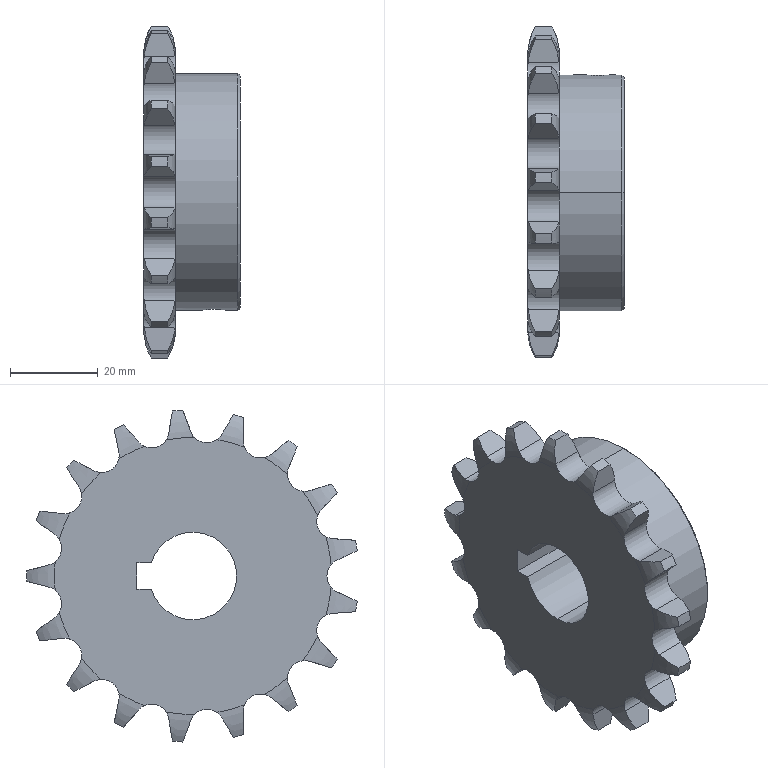Part | STEP file | RS40-1B17T-SS-H20_with key | 1 solid | 122 faces | box 22 x 75.554 x 75.859 mm | volume 50736 mm3 | cylinder 43 | plane 41 | torus 36 | cone 2 | commonest cylinder face diameters 7.92 x17 76 x17 6 x4 20 x3 54 x2